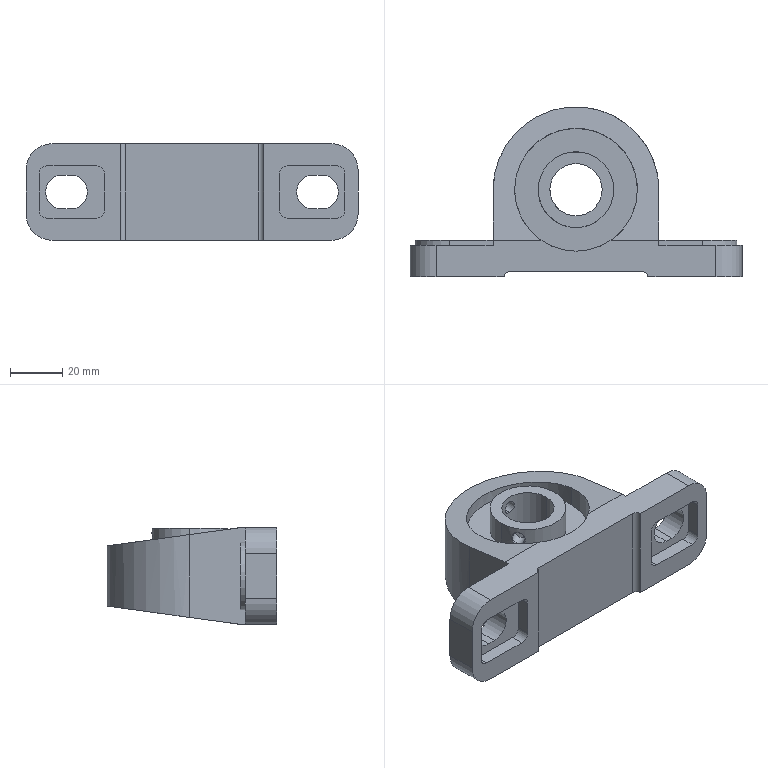Part | SolidWorks | features BaseBody 1 | 1 solid | 76 faces | box 127 x 65 x 37 mm | volume 109868 mm3 | plane 37 | cylinder 35 | cone 4 | commonest cylinder face diameters 6 x8 20 x6 4.917 x4 13 x4 29 x4 47 x4